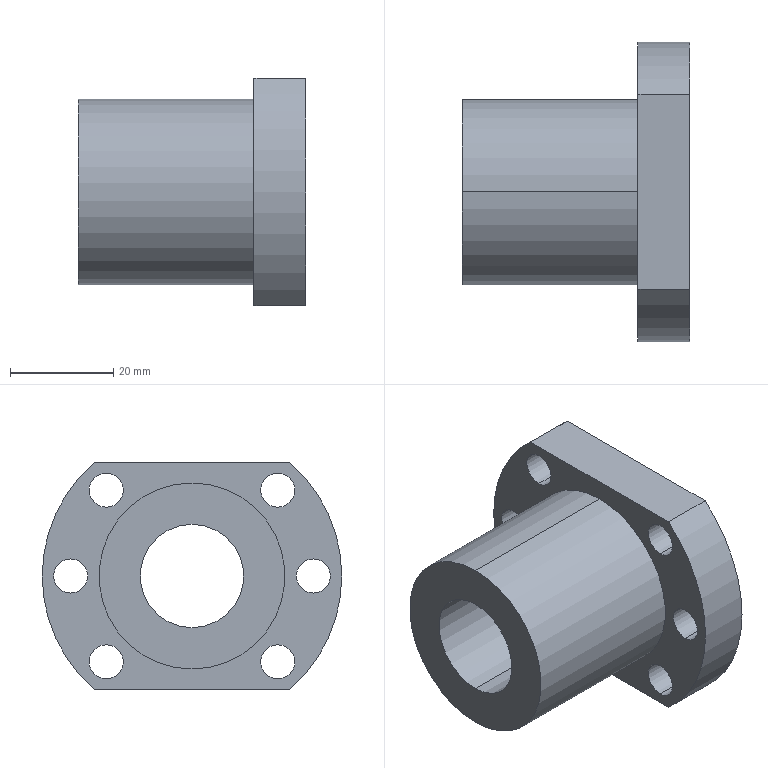Part | STEP file | PN_0026 20-5T3 nut | 1 solid | 23 faces | box 44 x 58 x 44 mm | volume 41531 mm3 | cylinder 18 | plane 5 | commonest cylinder face diameters 6.6 x12 20 x2 36 x2 58 x2